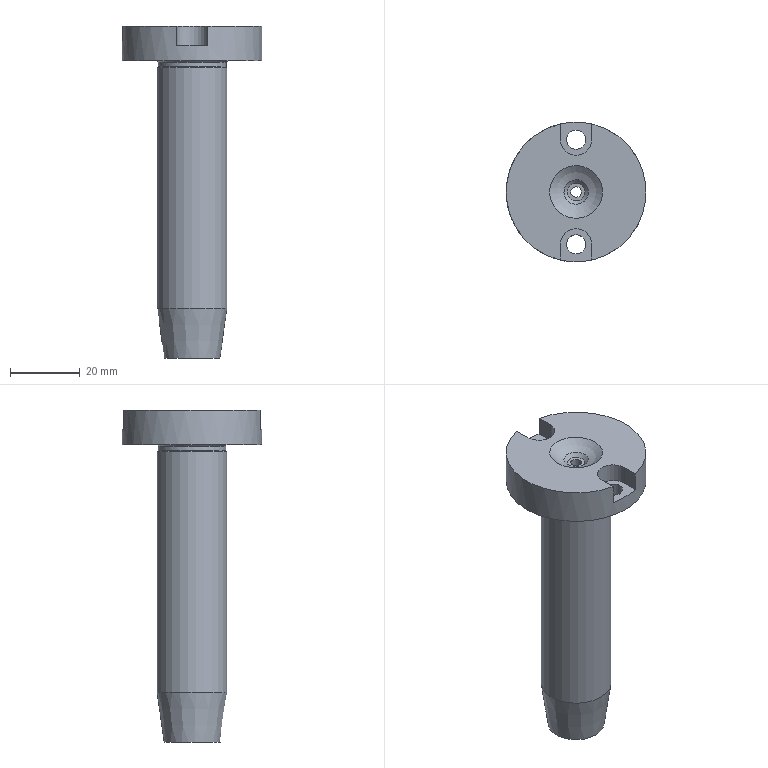Part | STEP file | 1_id706_xmt_txt | 1 solid | 23 faces | box 40 x 40 x 95 mm | volume 34804 mm3 | plane 10 | cylinder 7 | cone 3 | torus 2 | sphere 1 | commonest cylinder face diameters 5.5 x2 9 x2 19.4 x1 20 x1 40 x1
STEP:
#1=CARTESIAN_POINT('',(4.5,70.513,191.));
#2=VERTEX_POINT('',#1);
#3=CARTESIAN_POINT('',(4.5,109.487,191.));
#4=VERTEX_POINT('',#3);
#5=CARTESIAN_POINT('',(0.,90.,191.));
#6=DIRECTION('',(0.,0.,1.));
#7=DIRECTION('',(-1.,0.,0.));
#8=AXIS2_PLACEMENT_3D('',#5,#6,#7);
#9=CIRCLE('',#8,20.);
#10=EDGE_CURVE('',#2,#4,#9,.T.);
#11=ORIENTED_EDGE('',*,*,#10,.F.);
#12=CARTESIAN_POINT('',(4.5,70.513,185.5));
#13=VERTEX_POINT('',#12);
#14=CARTESIAN_POINT('',(4.5,70.513,188.25));
#15=DIRECTION('',(0.,0.,-1.));
#16=VECTOR('',#15,1.);
#17=LINE('',#14,#16);
#18=EDGE_CURVE('',#2,#13,#17,.T.);
#19=ORIENTED_EDGE('',*,*,#18,.T.);
#20=CARTESIAN_POINT('',(-4.5,70.513,185.5));
#21=VERTEX_POINT('',#20);
#22=CARTESIAN_POINT('',(0.,90.,185.5));
#23=DIRECTION('',(0.,0.,-1.));
#24=DIRECTION('',(-1.,0.,0.));
#25=AXIS2_PLACEMENT_3D('',#22,#23,#24);
#26=CIRCLE('',#25,20.);
#27=EDGE_CURVE('',#13,#21,#26,.T.);
#28=ORIENTED_EDGE('',*,*,#27,.T.);
#29=CARTESIAN_POINT('',(-4.5,70.513,191.));
#30=VERTEX_POINT('',#29);
#31=CARTESIAN_POINT('',(-4.5,70.513,188.25));
#32=DIRECTION('',(0.,0.,1.));
#33=VECTOR('',#32,1.);
#34=LINE('',#31,#33);
#35=EDGE_CURVE('',#21,#30,#34,.T.);
#36=ORIENTED_EDGE('',*,*,#35,.T.);
#37=CARTESIAN_POINT('',(-4.5,109.487,191.));
#38=VERTEX_POINT('',#37);
#39=CARTESIAN_POINT('',(0.,90.,191.));
#40=DIRECTION('',(0.,0.,1.));
#41=DIRECTION('',(-1.,0.,0.));
#42=AXIS2_PLACEMENT_3D('',#39,#40,#41);
#43=CIRCLE('',#42,20.);
#44=EDGE_CURVE('',#38,#30,#43,.T.);
#45=ORIENTED_EDGE('',*,*,#44,.F.);
#46=CARTESIAN_POINT('',(-4.5,109.487,185.5));
#47=VERTEX_POINT('',#46);
#48=CARTESIAN_POINT('',(-4.5,109.487,188.25));
#49=DIRECTION('',(0.,0.,-1.));
#50=VECTOR('',#49,1.);
#51=LINE('',#48,#50);
#52=EDGE_CURVE('',#38,#47,#51,.T.);
#53=ORIENTED_EDGE('',*,*,#52,.T.);
#54=CARTESIAN_POINT('',(4.5,109.487,185.5));
#55=VERTEX_POINT('',#54);
#56=CARTESIAN_POINT('',(0.,90.,185.5));
#57=DIRECTION('',(0.,0.,-1.));
#58=DIRECTION('',(-1.,0.,0.));
#59=AXIS2_PLACEMENT_3D('',#56,#57,#58);
#60=CIRCLE('',#59,20.);
#61=EDGE_CURVE('',#47,#55,#60,.T.);
#62=ORIENTED_EDGE('',*,*,#61,.T.);
#63=CARTESIAN_POINT('',(4.5,109.487,188.25));
#64=DIRECTION('',(0.,0.,1.));
#65=VECTOR('',#64,1.);
#66=LINE('',#63,#65);
#67=EDGE_CURVE('',#55,#4,#66,.T.);
#68=ORIENTED_EDGE('',*,*,#67,.T.);
#69=EDGE_LOOP('',(#11,#19,#28,#36,#45,#53,#62,#68));
#70=FACE_BOUND('',#69,.T.);
#71=CARTESIAN_POINT('',(-20.,90.,181.));
#72=VERTEX_POINT('',#71);
#73=CARTESIAN_POINT('',(0.,90.,181.));
#74=DIRECTION('',(0.,0.,-1.));
#75=DIRECTION('',(-1.,0.,0.));
#76=AXIS2_PLACEMENT_3D('',#73,#74,#75);
#77=CIRCLE('',#76,20.);
#78=EDGE_CURVE('',#72,#72,#77,.T.);
#79=ORIENTED_EDGE('',*,*,#78,.F.);
#80=EDGE_LOOP('',(#79));
#81=FACE_BOUND('',#80,.T.);
#82=CARTESIAN_POINT('',(0.,90.,186.));
#83=DIRECTION('',(0.,0.,-1.));
#84=DIRECTION('',(1.,0.,0.));
#85=AXIS2_PLACEMENT_3D('',#82,#83,#84);
#86=CYLINDRICAL_SURFACE('',#85,20.);
#87=ADVANCED_FACE('',(#70,#81),#86,.T.);
#88=CARTESIAN_POINT('',(2.75,75.,181.));
#89=VERTEX_POINT('',#88);
#90=CARTESIAN_POINT('',(0.,75.,181.));
#91=DIRECTION('',(0.,0.,1.));
#92=DIRECTION('',(1.,0.,0.));
#93=AXIS2_PLACEMENT_3D('',#90,#91,#92);
#94=CIRCLE('',#93,2.75);
#95=EDGE_CURVE('',#89,#89,#94,.T.);
#96=ORIENTED_EDGE('',*,*,#95,.F.);
#97=EDGE_LOOP('',(#96));
#98=FACE_BOUND('',#97,.T.);
#99=CARTESIAN_POINT('',(2.75,75.,185.5));
#100=VERTEX_POINT('',#99);
#101=CARTESIAN_POINT('',(0.,75.,185.5));
#102=DIRECTION('',(0.,0.,1.));
#103=DIRECTION('',(1.,0.,0.));
#104=AXIS2_PLACEMENT_3D('',#101,#102,#103);
#105=CIRCLE('',#104,2.75);
#106=EDGE_CURVE('',#100,#100,#105,.T.);
#107=ORIENTED_EDGE('',*,*,#106,.T.);
#108=EDGE_LOOP('',(#107));
#109=FACE_BOUND('',#108,.T.);
#110=CARTESIAN_POINT('',(0.,75.,186.));
#111=DIRECTION('',(0.,0.,-1.));
#112=DIRECTION('',(-1.,0.,0.));
#113=AXIS2_PLACEMENT_3D('',#110,#111,#112);
#114=CYLINDRICAL_SURFACE('',#113,2.75);
#115=ADVANCED_FACE('',(#98,#109),#114,.F.);
#116=CARTESIAN_POINT('',(-2.75,105.,181.));
#117=VERTEX_POINT('',#116);
#118=CARTESIAN_POINT('',(0.,105.,181.));
#119=DIRECTION('',(0.,0.,1.));
#120=DIRECTION('',(-1.,0.,0.));
#121=AXIS2_PLACEMENT_3D('',#118,#119,#120);
#122=CIRCLE('',#121,2.75);
#123=EDGE_CURVE('',#117,#117,#122,.T.);
#124=ORIENTED_EDGE('',*,*,#123,.F.);
#125=EDGE_LOOP('',(#124));
#126=FACE_BOUND('',#125,.T.);
#127=CARTESIAN_POINT('',(-2.75,105.,185.5));
#128=VERTEX_POINT('',#127);
#129=CARTESIAN_POINT('',(0.,105.,185.5));
#130=DIRECTION('',(0.,0.,1.));
#131=DIRECTION('',(-1.,0.,0.));
#132=AXIS2_PLACEMENT_3D('',#129,#130,#131);
#133=CIRCLE('',#132,2.75);
#134=EDGE_CURVE('',#128,#128,#133,.T.);
#135=ORIENTED_EDGE('',*,*,#134,.T.);
#136=EDGE_LOOP('',(#135));
#137=FACE_BOUND('',#136,.T.);
#138=CARTESIAN_POINT('',(0.,105.,186.));
#139=DIRECTION('',(0.,0.,-1.));
#140=DIRECTION('',(1.,0.,0.));
#141=AXIS2_PLACEMENT_3D('',#138,#139,#140);
#142=CYLINDRICAL_SURFACE('',#141,2.75);
#143=ADVANCED_FACE('',(#126,#137),#142,.F.);
#144=CARTESIAN_POINT('',(0.,100.,110.231));
#145=VERTEX_POINT('',#144);
#146=CARTESIAN_POINT('',(0.,90.,110.231));
#147=DIRECTION('',(0.,0.,1.));
#148=DIRECTION('',(0.,1.,0.));
#149=AXIS2_PLACEMENT_3D('',#146,#147,#148);
#150=CIRCLE('',#149,10.);
#151=EDGE_CURVE('',#145,#145,#150,.T.);
#152=ORIENTED_EDGE('',*,*,#151,.T.);
#153=EDGE_LOOP('',(#152));
#154=FACE_BOUND('',#153,.T.);
#155=CARTESIAN_POINT('',(0.,100.,179.));
#156=VERTEX_POINT('',#155);
#157=CARTESIAN_POINT('',(0.,90.,179.));
#158=DIRECTION('',(0.,0.,-1.));
#159=DIRECTION('',(0.,1.,0.));
#160=AXIS2_PLACEMENT_3D('',#157,#158,#159);
#161=CIRCLE('',#160,10.);
#162=EDGE_CURVE('',#156,#156,#161,.T.);
#163=ORIENTED_EDGE('',*,*,#162,.T.);
#164=EDGE_LOOP('',(#163));
#165=FACE_BOUND('',#164,.T.);
#166=CARTESIAN_POINT('',(0.,90.,145.615));
#167=DIRECTION('',(0.,0.,1.));
#168=DIRECTION('',(0.,-1.,0.));
#169=AXIS2_PLACEMENT_3D('',#166,#167,#168);
#170=CYLINDRICAL_SURFACE('',#169,10.);
#171=ADVANCED_FACE('',(#154,#165),#170,.T.);
#172=CARTESIAN_POINT('',(0.,98.,96.));
#173=VERTEX_POINT('',#172);
#174=CARTESIAN_POINT('',(0.,90.,96.));
#175=DIRECTION('',(0.,0.,1.));
#176=DIRECTION('',(0.,1.,0.));
#177=AXIS2_PLACEMENT_3D('',#174,#175,#176);
#178=CIRCLE('',#177,8.);
#179=EDGE_CURVE('',#173,#173,#178,.T.);
#180=ORIENTED_EDGE('',*,*,#179,.T.);
#181=EDGE_LOOP('',(#180));
#182=FACE_BOUND('',#181,.T.);
#183=ORIENTED_EDGE('',*,*,#151,.F.);
#184=EDGE_LOOP('',(#183));
#185=FACE_BOUND('',#184,.T.);
#186=CARTESIAN_POINT('',(0.,90.,103.115));
#187=DIRECTION('',(0.,0.,1.));
#188=DIRECTION('',(0.,-1.,0.));
#189=AXIS2_PLACEMENT_3D('',#186,#187,#188);
#190=CONICAL_SURFACE('',#189,9.,8.);
#191=ADVANCED_FACE('',(#182,#185),#190,.T.);
#192=CARTESIAN_POINT('',(-2.5,90.,187.5));
#193=VERTEX_POINT('',#192);
#194=CARTESIAN_POINT('',(0.,90.,187.5));
#195=DIRECTION('',(0.,0.,-1.));
#196=DIRECTION('',(-1.,0.,0.));
#197=AXIS2_PLACEMENT_3D('',#194,#195,#196);
#198=CIRCLE('',#197,2.5);
#199=EDGE_CURVE('',#193,#193,#198,.T.);
#200=ORIENTED_EDGE('',*,*,#199,.T.);
#201=EDGE_LOOP('',(#200));
#202=FACE_BOUND('',#201,.T.);
#203=CARTESIAN_POINT('',(-3.5,90.,188.572));
#204=VERTEX_POINT('',#203);
#205=CARTESIAN_POINT('',(0.,90.,188.572));
#206=DIRECTION('',(0.,0.,1.));
#207=DIRECTION('',(-1.,0.,0.));
#208=AXIS2_PLACEMENT_3D('',#205,#206,#207);
#209=CIRCLE('',#208,3.5);
#210=EDGE_CURVE('',#204,#204,#209,.T.);
#211=ORIENTED_EDGE('',*,*,#210,.T.);
#212=EDGE_LOOP('',(#211));
#213=FACE_BOUND('',#212,.T.);
#214=CARTESIAN_POINT('',(0.,90.,188.036));
#215=DIRECTION('',(0.,0.,1.));
#216=DIRECTION('',(1.,0.,0.));
#217=AXIS2_PLACEMENT_3D('',#214,#215,#216);
#218=CONICAL_SURFACE('',#217,3.,43.019);
#219=ADVANCED_FACE('',(#202,#213),#218,.F.);
#220=ORIENTED_EDGE('',*,*,#210,.F.);
#221=EDGE_LOOP('',(#220));
#222=FACE_BOUND('',#221,.T.);
#223=CARTESIAN_POINT('',(0.,82.45,191.));
#224=VERTEX_POINT('',#223);
#225=CARTESIAN_POINT('',(0.,90.,191.));
#226=DIRECTION('',(0.,0.,-1.));
#227=DIRECTION('',(0.,-1.,0.));
#228=AXIS2_PLACEMENT_3D('',#225,#226,#227);
#229=CIRCLE('',#228,7.55);
#230=EDGE_CURVE('',#224,#224,#229,.T.);
#231=ORIENTED_EDGE('',*,*,#230,.F.);
#232=EDGE_LOOP('',(#231));
#233=FACE_BOUND('',#232,.T.);
#234=CARTESIAN_POINT('',(0.,90.,199.));
#235=DIRECTION('',(0.,0.,-1.));
#236=DIRECTION('',(1.,0.,0.));
#237=AXIS2_PLACEMENT_3D('',#234,#235,#236);
#238=SPHERICAL_SURFACE('',#237,11.);
#239=ADVANCED_FACE('',(#222,#233),#238,.F.);
#240=CARTESIAN_POINT('',(-3.912,90.,96.));
#241=VERTEX_POINT('',#240);
#242=CARTESIAN_POINT('',(0.,90.,96.));
#243=DIRECTION('',(0.,0.,1.));
#244=DIRECTION('',(-1.,0.,0.));
#245=AXIS2_PLACEMENT_3D('',#242,#243,#244);
#246=CIRCLE('',#245,3.912);
#247=EDGE_CURVE('',#241,#241,#246,.T.);
#248=ORIENTED_EDGE('',*,*,#247,.F.);
#249=EDGE_LOOP('',(#248));
#250=FACE_BOUND('',#249,.T.);
#251=CARTESIAN_POINT('',(-1.516,90.,187.5));
#252=VERTEX_POINT('',#251);
#253=CARTESIAN_POINT('',(0.,90.,187.5));
#254=DIRECTION('',(0.,0.,-1.));
#255=DIRECTION('',(-1.,0.,0.));
#256=AXIS2_PLACEMENT_3D('',#253,#254,#255);
#257=CIRCLE('',#256,1.516);
#258=EDGE_CURVE('',#252,#252,#257,.T.);
#259=ORIENTED_EDGE('',*,*,#258,.F.);
#260=EDGE_LOOP('',(#259));
#261=FACE_BOUND('',#260,.T.);
#262=CARTESIAN_POINT('',(0.,90.,142.051));
#263=DIRECTION('',(0.,0.,-1.));
#264=DIRECTION('',(1.,0.,0.));
#265=AXIS2_PLACEMENT_3D('',#262,#263,#264);
#266=CONICAL_SURFACE('',#265,2.706,1.5);
#267=ADVANCED_FACE('',(#250,#261),#266,.F.);
#268=CARTESIAN_POINT('',(10.2,90.,181.));
#269=VERTEX_POINT('',#268);
#270=CARTESIAN_POINT('',(0.,90.,181.));
#271=DIRECTION('',(0.,0.,-1.));
#272=DIRECTION('',(1.,0.,0.));
#273=AXIS2_PLACEMENT_3D('',#270,#271,#272);
#274=CIRCLE('',#273,10.2);
#275=EDGE_CURVE('',#269,#269,#274,.T.);
#276=ORIENTED_EDGE('',*,*,#275,.T.);
#277=EDGE_LOOP('',(#276));
#278=FACE_BOUND('',#277,.T.);
#279=CARTESIAN_POINT('',(9.7,90.,180.5));
#280=VERTEX_POINT('',#279);
#281=CARTESIAN_POINT('',(0.,90.,180.5));
#282=DIRECTION('',(0.,0.,1.));
#283=DIRECTION('',(1.,0.,0.));
#284=AXIS2_PLACEMENT_3D('',#281,#282,#283);
#285=CIRCLE('',#284,9.7);
#286=EDGE_CURVE('',#280,#280,#285,.T.);
#287=ORIENTED_EDGE('',*,*,#286,.T.);
#288=EDGE_LOOP('',(#287));
#289=FACE_BOUND('',#288,.T.);
#290=CARTESIAN_POINT('',(0.,90.,180.5));
#291=DIRECTION('',(0.,0.,-1.));
#292=DIRECTION('',(1.,0.,0.));
#293=AXIS2_PLACEMENT_3D('',#290,#291,#292);
#294=TOROIDAL_SURFACE('',#293,10.2,0.5);
#295=ADVANCED_FACE('',(#278,#289),#294,.F.);
#296=ORIENTED_EDGE('',*,*,#286,.F.);
#297=EDGE_LOOP('',(#296));
#298=FACE_BOUND('',#297,.T.);
#299=CARTESIAN_POINT('',(9.7,90.,179.3));
#300=VERTEX_POINT('',#299);
#301=CARTESIAN_POINT('',(0.,90.,179.3));
#302=DIRECTION('',(0.,0.,-1.));
#303=DIRECTION('',(1.,0.,0.));
#304=AXIS2_PLACEMENT_3D('',#301,#302,#303);
#305=CIRCLE('',#304,9.7);
#306=EDGE_CURVE('',#300,#300,#305,.T.);
#307=ORIENTED_EDGE('',*,*,#306,.F.);
#308=EDGE_LOOP('',(#307));
#309=FACE_BOUND('',#308,.T.);
#310=CARTESIAN_POINT('',(0.,90.,180.));
#311=DIRECTION('',(0.,0.,-1.));
#312=DIRECTION('',(1.,0.,0.));
#313=AXIS2_PLACEMENT_3D('',#310,#311,#312);
#314=CYLINDRICAL_SURFACE('',#313,9.7);
#315=ADVANCED_FACE('',(#298,#309),#314,.T.);
#316=ORIENTED_EDGE('',*,*,#162,.F.);
#317=EDGE_LOOP('',(#316));
#318=FACE_BOUND('',#317,.T.);
#319=ORIENTED_EDGE('',*,*,#306,.T.);
#320=EDGE_LOOP('',(#319));
#321=FACE_BOUND('',#320,.T.);
#322=CARTESIAN_POINT('',(0.,90.,179.3));
#323=DIRECTION('',(0.,0.,1.));
#324=DIRECTION('',(-1.,0.,0.));
#325=AXIS2_PLACEMENT_3D('',#322,#323,#324);
#326=TOROIDAL_SURFACE('',#325,10.,0.3);
#327=ADVANCED_FACE('',(#318,#321),#326,.F.);
#328=ORIENTED_EDGE('',*,*,#123,.T.);
#329=EDGE_LOOP('',(#328));
#330=FACE_BOUND('',#329,.T.);
#331=ORIENTED_EDGE('',*,*,#95,.T.);
#332=EDGE_LOOP('',(#331));
#333=FACE_BOUND('',#332,.T.);
#334=ORIENTED_EDGE('',*,*,#78,.T.);
#335=EDGE_LOOP('',(#334));
#336=FACE_BOUND('',#335,.T.);
#337=ORIENTED_EDGE('',*,*,#275,.F.);
#338=EDGE_LOOP('',(#337));
#339=FACE_BOUND('',#338,.T.);
#340=CARTESIAN_POINT('',(0.,90.,181.));
#341=DIRECTION('',(0.,0.,-1.));
#342=DIRECTION('',(1.,0.,0.));
#343=AXIS2_PLACEMENT_3D('',#340,#341,#342);
#344=PLANE('',#343);
#345=ADVANCED_FACE('',(#330,#333,#336,#339),#344,.T.);
#346=ORIENTED_EDGE('',*,*,#258,.T.);
#347=EDGE_LOOP('',(#346));
#348=FACE_BOUND('',#347,.T.);
#349=ORIENTED_EDGE('',*,*,#199,.F.);
#350=EDGE_LOOP('',(#349));
#351=FACE_BOUND('',#350,.T.);
#352=CARTESIAN_POINT('',(0.,90.,187.5));
#353=DIRECTION('',(0.,0.,-1.));
#354=DIRECTION('',(1.,0.,0.));
#355=AXIS2_PLACEMENT_3D('',#352,#353,#354);
#356=PLANE('',#355);
#357=ADVANCED_FACE('',(#348,#351),#356,.F.);
#358=ORIENTED_EDGE('',*,*,#247,.T.);
#359=EDGE_LOOP('',(#358));
#360=FACE_BOUND('',#359,.T.);
#361=ORIENTED_EDGE('',*,*,#179,.F.);
#362=EDGE_LOOP('',(#361));
#363=FACE_BOUND('',#362,.T.);
#364=CARTESIAN_POINT('',(0.,94.,96.));
#365=DIRECTION('',(0.,0.,-1.));
#366=DIRECTION('',(0.,1.,0.));
#367=AXIS2_PLACEMENT_3D('',#364,#365,#366);
#368=PLANE('',#367);
#369=ADVANCED_FACE('',(#360,#363),#368,.T.);
#370=ORIENTED_EDGE('',*,*,#61,.F.);
#371=CARTESIAN_POINT('',(-4.5,105.,185.5));
#372=VERTEX_POINT('',#371);
#373=CARTESIAN_POINT('',(-4.5,122.5,185.5));
#374=DIRECTION('',(0.,1.,0.));
#375=VECTOR('',#374,1.);
#376=LINE('',#373,#375);
#377=EDGE_CURVE('',#372,#47,#376,.T.);
#378=ORIENTED_EDGE('',*,*,#377,.F.);
#379=CARTESIAN_POINT('',(4.5,105.,185.5));
#380=VERTEX_POINT('',#379);
#381=CARTESIAN_POINT('',(0.,105.,185.5));
#382=DIRECTION('',(0.,0.,-1.));
#383=DIRECTION('',(-1.,0.,0.));
#384=AXIS2_PLACEMENT_3D('',#381,#382,#383);
#385=CIRCLE('',#384,4.5);
#386=EDGE_CURVE('',#380,#372,#385,.T.);
#387=ORIENTED_EDGE('',*,*,#386,.F.);
#388=CARTESIAN_POINT('',(4.5,122.5,185.5));
#389=DIRECTION('',(0.,-1.,0.));
#390=VECTOR('',#389,1.);
#391=LINE('',#388,#390);
#392=EDGE_CURVE('',#55,#380,#391,.T.);
#393=ORIENTED_EDGE('',*,*,#392,.F.);
#394=EDGE_LOOP('',(#370,#378,#387,#393));
#395=FACE_BOUND('',#394,.T.);
#396=ORIENTED_EDGE('',*,*,#134,.F.);
#397=EDGE_LOOP('',(#396));
#398=FACE_BOUND('',#397,.T.);
#399=CARTESIAN_POINT('',(0.,122.5,185.5));
#400=DIRECTION('',(0.,0.,-1.));
#401=DIRECTION('',(1.,0.,0.));
#402=AXIS2_PLACEMENT_3D('',#399,#400,#401);
#403=PLANE('',#402);
#404=ADVANCED_FACE('',(#395,#398),#403,.F.);
#405=ORIENTED_EDGE('',*,*,#67,.F.);
#406=ORIENTED_EDGE('',*,*,#392,.T.);
#407=CARTESIAN_POINT('',(4.5,105.,191.));
#408=VERTEX_POINT('',#407);
#409=CARTESIAN_POINT('',(4.5,105.,188.25));
#410=DIRECTION('',(0.,0.,1.));
#411=VECTOR('',#410,1.);
#412=LINE('',#409,#411);
#413=EDGE_CURVE('',#380,#408,#412,.T.);
#414=ORIENTED_EDGE('',*,*,#413,.T.);
#415=CARTESIAN_POINT('',(4.5,106.25,191.));
#416=DIRECTION('',(0.,-1.,0.));
#417=VECTOR('',#416,1.);
#418=LINE('',#415,#417);
#419=EDGE_CURVE('',#4,#408,#418,.T.);
#420=ORIENTED_EDGE('',*,*,#419,.F.);
#421=EDGE_LOOP('',(#405,#406,#414,#420));
#422=FACE_OUTER_BOUND('',#421,.T.);
#423=CARTESIAN_POINT('',(4.5,122.5,188.25));
#424=DIRECTION('',(-1.,0.,0.));
#425=DIRECTION('',(0.,0.,-1.));
#426=AXIS2_PLACEMENT_3D('',#423,#424,#425);
#427=PLANE('',#426);
#428=ADVANCED_FACE('',(#422),#427,.T.);
#429=ORIENTED_EDGE('',*,*,#413,.F.);
#430=ORIENTED_EDGE('',*,*,#386,.T.);
#431=CARTESIAN_POINT('',(-4.5,105.,191.));
#432=VERTEX_POINT('',#431);
#433=CARTESIAN_POINT('',(-4.5,105.,188.25));
#434=DIRECTION('',(0.,0.,1.));
#435=VECTOR('',#434,1.);
#436=LINE('',#433,#435);
#437=EDGE_CURVE('',#372,#432,#436,.T.);
#438=ORIENTED_EDGE('',*,*,#437,.T.);
#439=CARTESIAN_POINT('',(0.,105.,191.));
#440=DIRECTION('',(0.,0.,-1.));
#441=DIRECTION('',(-1.,0.,0.));
#442=AXIS2_PLACEMENT_3D('',#439,#440,#441);
#443=CIRCLE('',#442,4.5);
#444=EDGE_CURVE('',#408,#432,#443,.T.);
#445=ORIENTED_EDGE('',*,*,#444,.F.);
#446=EDGE_LOOP('',(#429,#430,#438,#445));
#447=FACE_OUTER_BOUND('',#446,.T.);
#448=CARTESIAN_POINT('',(0.,105.,188.25));
#449=DIRECTION('',(0.,0.,-1.));
#450=DIRECTION('',(1.,0.,0.));
#451=AXIS2_PLACEMENT_3D('',#448,#449,#450);
#452=CYLINDRICAL_SURFACE('',#451,4.5);
#453=ADVANCED_FACE('',(#447),#452,.F.);
#454=ORIENTED_EDGE('',*,*,#52,.F.);
#455=CARTESIAN_POINT('',(-4.5,106.25,191.));
#456=DIRECTION('',(0.,1.,0.));
#457=VECTOR('',#456,1.);
#458=LINE('',#455,#457);
#459=EDGE_CURVE('',#432,#38,#458,.T.);
#460=ORIENTED_EDGE('',*,*,#459,.F.);
#461=ORIENTED_EDGE('',*,*,#437,.F.);
#462=ORIENTED_EDGE('',*,*,#377,.T.);
#463=EDGE_LOOP('',(#454,#460,#461,#462));
#464=FACE_OUTER_BOUND('',#463,.T.);
#465=CARTESIAN_POINT('',(-4.5,122.5,188.25));
#466=DIRECTION('',(1.,0.,0.));
#467=DIRECTION('',(0.,0.,1.));
#468=AXIS2_PLACEMENT_3D('',#465,#466,#467);
#469=PLANE('',#468);
#470=ADVANCED_FACE('',(#464),#469,.T.);
#471=ORIENTED_EDGE('',*,*,#27,.F.);
#472=CARTESIAN_POINT('',(4.5,75.,185.5));
#473=VERTEX_POINT('',#472);
#474=CARTESIAN_POINT('',(4.5,57.5,185.5));
#475=DIRECTION('',(0.,-1.,0.));
#476=VECTOR('',#475,1.);
#477=LINE('',#474,#476);
#478=EDGE_CURVE('',#473,#13,#477,.T.);
#479=ORIENTED_EDGE('',*,*,#478,.F.);
#480=CARTESIAN_POINT('',(-4.5,75.,185.5));
#481=VERTEX_POINT('',#480);
#482=CARTESIAN_POINT('',(0.,75.,185.5));
#483=DIRECTION('',(0.,0.,-1.));
#484=DIRECTION('',(1.,0.,0.));
#485=AXIS2_PLACEMENT_3D('',#482,#483,#484);
#486=CIRCLE('',#485,4.5);
#487=EDGE_CURVE('',#481,#473,#486,.T.);
#488=ORIENTED_EDGE('',*,*,#487,.F.);
#489=CARTESIAN_POINT('',(-4.5,57.5,185.5));
#490=DIRECTION('',(0.,1.,0.));
#491=VECTOR('',#490,1.);
#492=LINE('',#489,#491);
#493=EDGE_CURVE('',#21,#481,#492,.T.);
#494=ORIENTED_EDGE('',*,*,#493,.F.);
#495=EDGE_LOOP('',(#471,#479,#488,#494));
#496=FACE_BOUND('',#495,.T.);
#497=ORIENTED_EDGE('',*,*,#106,.F.);
#498=EDGE_LOOP('',(#497));
#499=FACE_BOUND('',#498,.T.);
#500=CARTESIAN_POINT('',(0.,57.5,185.5));
#501=DIRECTION('',(0.,0.,-1.));
#502=DIRECTION('',(-1.,0.,0.));
#503=AXIS2_PLACEMENT_3D('',#500,#501,#502);
#504=PLANE('',#503);
#505=ADVANCED_FACE('',(#496,#499),#504,.F.);
#506=ORIENTED_EDGE('',*,*,#35,.F.);
#507=ORIENTED_EDGE('',*,*,#493,.T.);
#508=CARTESIAN_POINT('',(-4.5,75.,191.));
#509=VERTEX_POINT('',#508);
#510=CARTESIAN_POINT('',(-4.5,75.,188.25));
#511=DIRECTION('',(0.,0.,1.));
#512=VECTOR('',#511,1.);
#513=LINE('',#510,#512);
#514=EDGE_CURVE('',#481,#509,#513,.T.);
#515=ORIENTED_EDGE('',*,*,#514,.T.);
#516=CARTESIAN_POINT('',(-4.5,73.75,191.));
#517=DIRECTION('',(0.,1.,0.));
#518=VECTOR('',#517,1.);
#519=LINE('',#516,#518);
#520=EDGE_CURVE('',#30,#509,#519,.T.);
#521=ORIENTED_EDGE('',*,*,#520,.F.);
#522=EDGE_LOOP('',(#506,#507,#515,#521));
#523=FACE_OUTER_BOUND('',#522,.T.);
#524=CARTESIAN_POINT('',(-4.5,57.5,188.25));
#525=DIRECTION('',(1.,0.,0.));
#526=DIRECTION('',(0.,0.,-1.));
#527=AXIS2_PLACEMENT_3D('',#524,#525,#526);
#528=PLANE('',#527);
#529=ADVANCED_FACE('',(#523),#528,.T.);
#530=ORIENTED_EDGE('',*,*,#514,.F.);
#531=ORIENTED_EDGE('',*,*,#487,.T.);
#532=CARTESIAN_POINT('',(4.5,75.,191.));
#533=VERTEX_POINT('',#532);
#534=CARTESIAN_POINT('',(4.5,75.,188.25));
#535=DIRECTION('',(0.,0.,1.));
#536=VECTOR('',#535,1.);
#537=LINE('',#534,#536);
#538=EDGE_CURVE('',#473,#533,#537,.T.);
#539=ORIENTED_EDGE('',*,*,#538,.T.);
#540=CARTESIAN_POINT('',(0.,75.,191.));
#541=DIRECTION('',(0.,0.,-1.));
#542=DIRECTION('',(1.,0.,0.));
#543=AXIS2_PLACEMENT_3D('',#540,#541,#542);
#544=CIRCLE('',#543,4.5);
#545=EDGE_CURVE('',#509,#533,#544,.T.);
#546=ORIENTED_EDGE('',*,*,#545,.F.);
#547=EDGE_LOOP('',(#530,#531,#539,#546));
#548=FACE_OUTER_BOUND('',#547,.T.);
#549=CARTESIAN_POINT('',(0.,75.,188.25));
#550=DIRECTION('',(0.,0.,-1.));
#551=DIRECTION('',(-1.,0.,0.));
#552=AXIS2_PLACEMENT_3D('',#549,#550,#551);
#553=CYLINDRICAL_SURFACE('',#552,4.5);
#554=ADVANCED_FACE('',(#548),#553,.F.);
#555=ORIENTED_EDGE('',*,*,#18,.F.);
#556=CARTESIAN_POINT('',(4.5,73.75,191.));
#557=DIRECTION('',(0.,-1.,0.));
#558=VECTOR('',#557,1.);
#559=LINE('',#556,#558);
#560=EDGE_CURVE('',#533,#2,#559,.T.);
#561=ORIENTED_EDGE('',*,*,#560,.F.);
#562=ORIENTED_EDGE('',*,*,#538,.F.);
#563=ORIENTED_EDGE('',*,*,#478,.T.);
#564=EDGE_LOOP('',(#555,#561,#562,#563));
#565=FACE_OUTER_BOUND('',#564,.T.);
#566=CARTESIAN_POINT('',(4.5,57.5,188.25));
#567=DIRECTION('',(-1.,0.,0.));
#568=DIRECTION('',(0.,0.,1.));
#569=AXIS2_PLACEMENT_3D('',#566,#567,#568);
#570=PLANE('',#569);
#571=ADVANCED_FACE('',(#565),#570,.T.);
#572=ORIENTED_EDGE('',*,*,#230,.T.);
#573=EDGE_LOOP('',(#572));
#574=FACE_BOUND('',#573,.T.);
#575=ORIENTED_EDGE('',*,*,#459,.T.);
#576=ORIENTED_EDGE('',*,*,#44,.T.);
#577=ORIENTED_EDGE('',*,*,#520,.T.);
#578=ORIENTED_EDGE('',*,*,#545,.T.);
#579=ORIENTED_EDGE('',*,*,#560,.T.);
#580=ORIENTED_EDGE('',*,*,#10,.T.);
#581=ORIENTED_EDGE('',*,*,#419,.T.);
#582=ORIENTED_EDGE('',*,*,#444,.T.);
#583=EDGE_LOOP('',(#575,#576,#577,#578,#579,#580,#581,#582));
#584=FACE_BOUND('',#583,.T.);
#585=CARTESIAN_POINT('',(0.,90.,191.));
#586=DIRECTION('',(0.,0.,1.));
#587=DIRECTION('',(-1.,0.,0.));
#588=AXIS2_PLACEMENT_3D('',#585,#586,#587);
#589=PLANE('',#588);
#590=ADVANCED_FACE('',(#574,#584),#589,.T.);
#591=CLOSED_SHELL('',(#87,#115,#143,#171,#191,#219,#239,#267,#295,#315,#327,#345,#357,#369,#404,#428,#453,#470,#505,#529,#554,#571,#590));
#592=MANIFOLD_SOLID_BREP('',#591);
#593=(LENGTH_UNIT()NAMED_UNIT(*)SI_UNIT(.MILLI.,.METRE.));
#594=UNCERTAINTY_MEASURE_WITH_UNIT(LENGTH_MEASURE(0.00002),#593,'','');
#595=(NAMED_UNIT(*)PLANE_ANGLE_UNIT()SI_UNIT($,.RADIAN.));
#596=PLANE_ANGLE_MEASURE_WITH_UNIT(PLANE_ANGLE_MEASURE(0.01745),#595);
#597=DIMENSIONAL_EXPONENTS(0.,0.,0.,0.,0.,0.,0.);
#598=(CONVERSION_BASED_UNIT('DEGREE',#596)NAMED_UNIT(#597)PLANE_ANGLE_UNIT());
#599=(NAMED_UNIT(*)SI_UNIT($,.STERADIAN.)SOLID_ANGLE_UNIT());
#600=(GEOMETRIC_REPRESENTATION_CONTEXT(3)GLOBAL_UNCERTAINTY_ASSIGNED_CONTEXT((#594))GLOBAL_UNIT_ASSIGNED_CONTEXT((#593,#598,#599))REPRESENTATION_CONTEXT('',''));
#601=ADVANCED_BREP_SHAPE_REPRESENTATION('',(#592),#600);